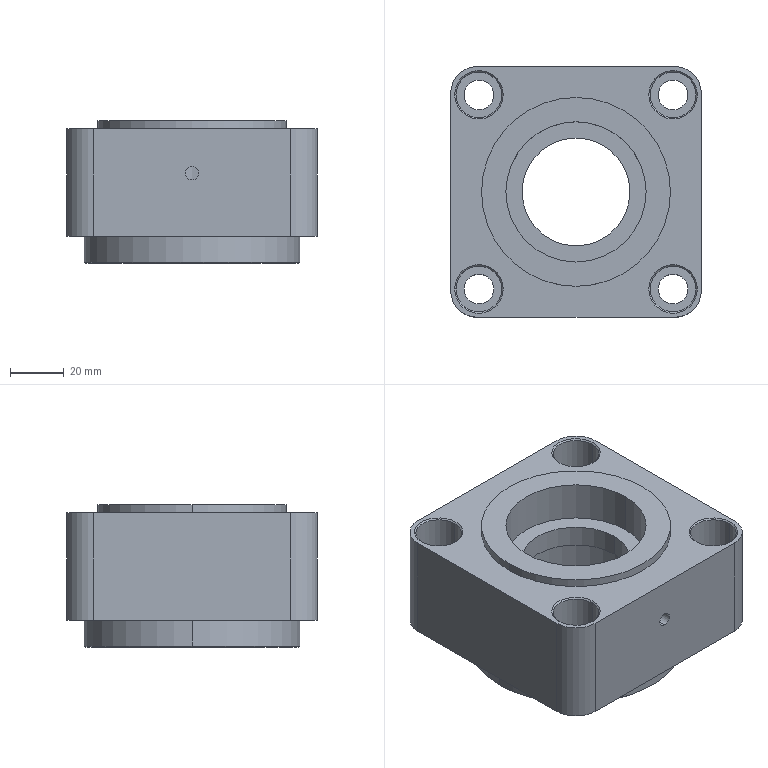Part | SolidWorks | features ICE 4, HoleWzd 3, BaseBody 1, MoveFace 1 | 1 solid | 73 faces | box 93 x 93 x 53 mm | volume 265876 mm3 | cylinder 41 | cone 18 | plane 14 | commonest cylinder face diameters 11 x8 17 x8 8.8 x5 2.5 x4 20 x4 52 x4